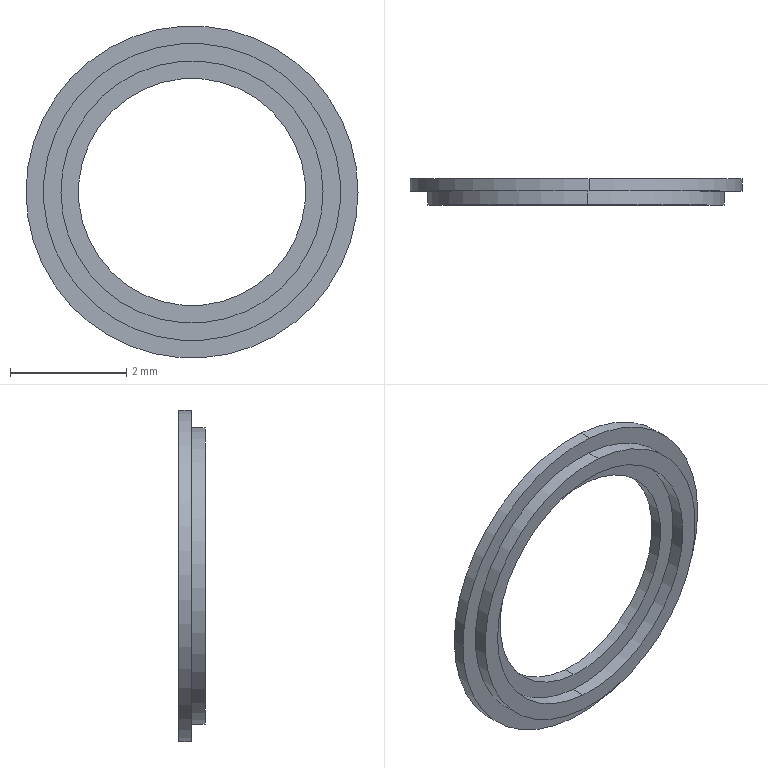Part | STEP file | 2026.6.15-Main Assembly图.sldasm-Part-192 | 1 solid | 12 faces | box 5.7 x 0.45 x 5.7 mm | volume 3.936 mm3 | cylinder 8 | plane 4 | commonest cylinder face diameters 3.9 x2 4.5 x2 5.1 x2 5.7 x2
STEP:
#1=CARTESIAN_POINT('',(-1557.488,1439.564,3405.544));
#2=VERTEX_POINT('',#1);
#3=CARTESIAN_POINT('',(-1557.088,1439.564,3410.628));
#4=VERTEX_POINT('',#3);
#5=CARTESIAN_POINT('',(-1557.288,1439.564,3408.086));
#6=DIRECTION('',(0.,1.,0.));
#7=DIRECTION('',(-0.0785,0.,-0.9969));
#8=AXIS2_PLACEMENT_3D('',#5,#6,#7);
#9=CIRCLE('',#8,2.55);
#10=EDGE_CURVE('',#2,#4,#9,.T.);
#11=ORIENTED_EDGE('',*,*,#10,.F.);
#12=CARTESIAN_POINT('',(-1557.288,1439.564,3408.086));
#13=DIRECTION('',(0.,1.,0.));
#14=DIRECTION('',(-0.0785,0.,-0.9969));
#15=AXIS2_PLACEMENT_3D('',#12,#13,#14);
#16=CIRCLE('',#15,2.55);
#17=EDGE_CURVE('',#4,#2,#16,.T.);
#18=ORIENTED_EDGE('',*,*,#17,.F.);
#19=EDGE_LOOP('',(#11,#18));
#20=FACE_OUTER_BOUND('',#19,.T.);
#21=CARTESIAN_POINT('',(-1557.465,1439.564,3405.843));
#22=VERTEX_POINT('',#21);
#23=CARTESIAN_POINT('',(-1557.112,1439.564,3410.329));
#24=VERTEX_POINT('',#23);
#25=CARTESIAN_POINT('',(-1557.288,1439.564,3408.086));
#26=DIRECTION('',(0.,1.,0.));
#27=DIRECTION('',(-0.0785,0.,-0.9969));
#28=AXIS2_PLACEMENT_3D('',#25,#26,#27);
#29=CIRCLE('',#28,2.25);
#30=EDGE_CURVE('',#22,#24,#29,.T.);
#31=ORIENTED_EDGE('',*,*,#30,.T.);
#32=CARTESIAN_POINT('',(-1557.288,1439.564,3408.086));
#33=DIRECTION('',(0.,1.,0.));
#34=DIRECTION('',(-0.0785,0.,-0.9969));
#35=AXIS2_PLACEMENT_3D('',#32,#33,#34);
#36=CIRCLE('',#35,2.25);
#37=EDGE_CURVE('',#24,#22,#36,.T.);
#38=ORIENTED_EDGE('',*,*,#37,.T.);
#39=EDGE_LOOP('',(#31,#38));
#40=FACE_BOUND('',#39,.T.);
#41=CARTESIAN_POINT('',(-1557.288,1439.564,3410.636));
#42=DIRECTION('',(0.,1.,0.));
#43=DIRECTION('',(1.,0.,0.));
#44=AXIS2_PLACEMENT_3D('',#41,#42,#43);
#45=PLANE('',#44);
#46=ADVANCED_FACE('',(#20,#40),#45,.F.);
#47=CARTESIAN_POINT('',(-1557.112,1439.804,3410.329));
#48=VERTEX_POINT('',#47);
#49=CARTESIAN_POINT('',(-1557.112,1459.814,3410.329));
#50=DIRECTION('',(0.,1.,0.));
#51=VECTOR('',#50,1000.);
#52=LINE('',#49,#51);
#53=EDGE_CURVE('',#24,#48,#52,.T.);
#54=ORIENTED_EDGE('',*,*,#53,.F.);
#55=ORIENTED_EDGE('',*,*,#30,.F.);
#56=CARTESIAN_POINT('',(-1557.465,1439.804,3405.843));
#57=VERTEX_POINT('',#56);
#58=CARTESIAN_POINT('',(-1557.465,1459.814,3405.843));
#59=DIRECTION('',(0.,1.,0.));
#60=VECTOR('',#59,1000.);
#61=LINE('',#58,#60);
#62=EDGE_CURVE('',#22,#57,#61,.T.);
#63=ORIENTED_EDGE('',*,*,#62,.T.);
#64=CARTESIAN_POINT('',(-1557.288,1439.804,3408.086));
#65=DIRECTION('',(0.,1.,0.));
#66=DIRECTION('',(-0.0785,0.,-0.9969));
#67=AXIS2_PLACEMENT_3D('',#64,#65,#66);
#68=CIRCLE('',#67,2.25);
#69=EDGE_CURVE('',#57,#48,#68,.T.);
#70=ORIENTED_EDGE('',*,*,#69,.T.);
#71=EDGE_LOOP('',(#54,#55,#63,#70));
#72=FACE_OUTER_BOUND('',#71,.T.);
#73=CARTESIAN_POINT('',(-1557.288,1459.814,3408.086));
#74=DIRECTION('',(0.,1.,0.));
#75=DIRECTION('',(0.0785,0.,0.9969));
#76=AXIS2_PLACEMENT_3D('',#73,#74,#75);
#77=CYLINDRICAL_SURFACE('',#76,2.25);
#78=ADVANCED_FACE('',(#72),#77,.F.);
#79=CARTESIAN_POINT('',(-1557.088,1439.804,3410.628));
#80=VERTEX_POINT('',#79);
#81=CARTESIAN_POINT('',(-1557.088,1459.814,3410.628));
#82=DIRECTION('',(0.,1.,0.));
#83=VECTOR('',#82,1000.);
#84=LINE('',#81,#83);
#85=EDGE_CURVE('',#4,#80,#84,.T.);
#86=ORIENTED_EDGE('',*,*,#85,.F.);
#87=ORIENTED_EDGE('',*,*,#17,.T.);
#88=CARTESIAN_POINT('',(-1557.488,1439.804,3405.544));
#89=VERTEX_POINT('',#88);
#90=CARTESIAN_POINT('',(-1557.488,1459.814,3405.544));
#91=DIRECTION('',(0.,1.,0.));
#92=VECTOR('',#91,1000.);
#93=LINE('',#90,#92);
#94=EDGE_CURVE('',#2,#89,#93,.T.);
#95=ORIENTED_EDGE('',*,*,#94,.T.);
#96=CARTESIAN_POINT('',(-1557.288,1439.804,3408.086));
#97=DIRECTION('',(0.,-1.,0.));
#98=DIRECTION('',(-0.0785,0.,-0.9969));
#99=AXIS2_PLACEMENT_3D('',#96,#97,#98);
#100=CIRCLE('',#99,2.55);
#101=EDGE_CURVE('',#89,#80,#100,.T.);
#102=ORIENTED_EDGE('',*,*,#101,.T.);
#103=EDGE_LOOP('',(#86,#87,#95,#102));
#104=FACE_OUTER_BOUND('',#103,.T.);
#105=CARTESIAN_POINT('',(-1557.288,1459.814,3408.086));
#106=DIRECTION('',(0.,1.,0.));
#107=DIRECTION('',(0.0785,0.,0.9969));
#108=AXIS2_PLACEMENT_3D('',#105,#106,#107);
#109=CYLINDRICAL_SURFACE('',#108,2.55);
#110=ADVANCED_FACE('',(#104),#109,.T.);
#111=ORIENTED_EDGE('',*,*,#69,.F.);
#112=CARTESIAN_POINT('',(-1557.288,1439.804,3408.086));
#113=DIRECTION('',(0.,1.,0.));
#114=DIRECTION('',(-0.0785,0.,-0.9969));
#115=AXIS2_PLACEMENT_3D('',#112,#113,#114);
#116=CIRCLE('',#115,2.25);
#117=EDGE_CURVE('',#48,#57,#116,.T.);
#118=ORIENTED_EDGE('',*,*,#117,.F.);
#119=EDGE_LOOP('',(#111,#118));
#120=FACE_OUTER_BOUND('',#119,.T.);
#121=CARTESIAN_POINT('',(-1557.441,1439.804,3406.142));
#122=VERTEX_POINT('',#121);
#123=CARTESIAN_POINT('',(-1557.135,1439.804,3410.03));
#124=VERTEX_POINT('',#123);
#125=CARTESIAN_POINT('',(-1557.288,1439.804,3408.086));
#126=DIRECTION('',(0.,1.,0.));
#127=DIRECTION('',(-0.0785,0.,-0.9969));
#128=AXIS2_PLACEMENT_3D('',#125,#126,#127);
#129=CIRCLE('',#128,1.95);
#130=EDGE_CURVE('',#122,#124,#129,.T.);
#131=ORIENTED_EDGE('',*,*,#130,.T.);
#132=CARTESIAN_POINT('',(-1557.288,1439.804,3408.086));
#133=DIRECTION('',(0.,1.,0.));
#134=DIRECTION('',(-0.0785,0.,-0.9969));
#135=AXIS2_PLACEMENT_3D('',#132,#133,#134);
#136=CIRCLE('',#135,1.95);
#137=EDGE_CURVE('',#124,#122,#136,.T.);
#138=ORIENTED_EDGE('',*,*,#137,.T.);
#139=EDGE_LOOP('',(#131,#138));
#140=FACE_BOUND('',#139,.T.);
#141=CARTESIAN_POINT('',(-1557.288,1439.804,3410.336));
#142=DIRECTION('',(0.,1.,0.));
#143=DIRECTION('',(1.,0.,0.));
#144=AXIS2_PLACEMENT_3D('',#141,#142,#143);
#145=PLANE('',#144);
#146=ADVANCED_FACE('',(#120,#140),#145,.F.);
#147=CARTESIAN_POINT('',(-1557.512,1439.804,3405.245));
#148=VERTEX_POINT('',#147);
#149=CARTESIAN_POINT('',(-1557.065,1439.804,3410.928));
#150=VERTEX_POINT('',#149);
#151=CARTESIAN_POINT('',(-1557.288,1439.804,3408.086));
#152=DIRECTION('',(0.,1.,0.));
#153=DIRECTION('',(-0.0785,0.,-0.9969));
#154=AXIS2_PLACEMENT_3D('',#151,#152,#153);
#155=CIRCLE('',#154,2.85);
#156=EDGE_CURVE('',#148,#150,#155,.T.);
#157=ORIENTED_EDGE('',*,*,#156,.F.);
#158=CARTESIAN_POINT('',(-1557.288,1439.804,3408.086));
#159=DIRECTION('',(0.,1.,0.));
#160=DIRECTION('',(-0.0785,0.,-0.9969));
#161=AXIS2_PLACEMENT_3D('',#158,#159,#160);
#162=CIRCLE('',#161,2.85);
#163=EDGE_CURVE('',#150,#148,#162,.T.);
#164=ORIENTED_EDGE('',*,*,#163,.F.);
#165=EDGE_LOOP('',(#157,#164));
#166=FACE_OUTER_BOUND('',#165,.T.);
#167=ORIENTED_EDGE('',*,*,#101,.F.);
#168=CARTESIAN_POINT('',(-1557.288,1439.804,3408.086));
#169=DIRECTION('',(0.,-1.,0.));
#170=DIRECTION('',(-0.0785,0.,-0.9969));
#171=AXIS2_PLACEMENT_3D('',#168,#169,#170);
#172=CIRCLE('',#171,2.55);
#173=EDGE_CURVE('',#80,#89,#172,.T.);
#174=ORIENTED_EDGE('',*,*,#173,.F.);
#175=EDGE_LOOP('',(#167,#174));
#176=FACE_BOUND('',#175,.T.);
#177=CARTESIAN_POINT('',(-1557.288,1439.804,3410.936));
#178=DIRECTION('',(0.,1.,0.));
#179=DIRECTION('',(1.,0.,0.));
#180=AXIS2_PLACEMENT_3D('',#177,#178,#179);
#181=PLANE('',#180);
#182=ADVANCED_FACE('',(#166,#176),#181,.F.);
#183=CARTESIAN_POINT('',(-1557.135,1440.014,3410.03));
#184=VERTEX_POINT('',#183);
#185=CARTESIAN_POINT('',(-1557.135,1459.814,3410.03));
#186=DIRECTION('',(0.,1.,0.));
#187=VECTOR('',#186,1000.);
#188=LINE('',#185,#187);
#189=EDGE_CURVE('',#124,#184,#188,.T.);
#190=ORIENTED_EDGE('',*,*,#189,.F.);
#191=ORIENTED_EDGE('',*,*,#130,.F.);
#192=CARTESIAN_POINT('',(-1557.441,1440.014,3406.142));
#193=VERTEX_POINT('',#192);
#194=CARTESIAN_POINT('',(-1557.441,1459.814,3406.142));
#195=DIRECTION('',(0.,1.,0.));
#196=VECTOR('',#195,1000.);
#197=LINE('',#194,#196);
#198=EDGE_CURVE('',#122,#193,#197,.T.);
#199=ORIENTED_EDGE('',*,*,#198,.T.);
#200=CARTESIAN_POINT('',(-1557.288,1440.014,3408.086));
#201=DIRECTION('',(0.,1.,0.));
#202=DIRECTION('',(-0.0785,0.,-0.9969));
#203=AXIS2_PLACEMENT_3D('',#200,#201,#202);
#204=CIRCLE('',#203,1.95);
#205=EDGE_CURVE('',#193,#184,#204,.T.);
#206=ORIENTED_EDGE('',*,*,#205,.T.);
#207=EDGE_LOOP('',(#190,#191,#199,#206));
#208=FACE_OUTER_BOUND('',#207,.T.);
#209=CARTESIAN_POINT('',(-1557.288,1459.814,3408.086));
#210=DIRECTION('',(0.,1.,0.));
#211=DIRECTION('',(0.0785,0.,0.9969));
#212=AXIS2_PLACEMENT_3D('',#209,#210,#211);
#213=CYLINDRICAL_SURFACE('',#212,1.95);
#214=ADVANCED_FACE('',(#208),#213,.F.);
#215=CARTESIAN_POINT('',(-1557.065,1440.014,3410.928));
#216=VERTEX_POINT('',#215);
#217=CARTESIAN_POINT('',(-1557.065,1459.814,3410.928));
#218=DIRECTION('',(0.,1.,0.));
#219=VECTOR('',#218,1000.);
#220=LINE('',#217,#219);
#221=EDGE_CURVE('',#150,#216,#220,.T.);
#222=ORIENTED_EDGE('',*,*,#221,.F.);
#223=ORIENTED_EDGE('',*,*,#163,.T.);
#224=CARTESIAN_POINT('',(-1557.512,1440.014,3405.245));
#225=VERTEX_POINT('',#224);
#226=CARTESIAN_POINT('',(-1557.512,1459.814,3405.245));
#227=DIRECTION('',(0.,1.,0.));
#228=VECTOR('',#227,1000.);
#229=LINE('',#226,#228);
#230=EDGE_CURVE('',#148,#225,#229,.T.);
#231=ORIENTED_EDGE('',*,*,#230,.T.);
#232=CARTESIAN_POINT('',(-1557.288,1440.014,3408.086));
#233=DIRECTION('',(0.,-1.,0.));
#234=DIRECTION('',(-0.0785,0.,-0.9969));
#235=AXIS2_PLACEMENT_3D('',#232,#233,#234);
#236=CIRCLE('',#235,2.85);
#237=EDGE_CURVE('',#225,#216,#236,.T.);
#238=ORIENTED_EDGE('',*,*,#237,.T.);
#239=EDGE_LOOP('',(#222,#223,#231,#238));
#240=FACE_OUTER_BOUND('',#239,.T.);
#241=CARTESIAN_POINT('',(-1557.288,1459.814,3408.086));
#242=DIRECTION('',(0.,1.,0.));
#243=DIRECTION('',(0.0785,0.,0.9969));
#244=AXIS2_PLACEMENT_3D('',#241,#242,#243);
#245=CYLINDRICAL_SURFACE('',#244,2.85);
#246=ADVANCED_FACE('',(#240),#245,.T.);
#247=ORIENTED_EDGE('',*,*,#237,.F.);
#248=CARTESIAN_POINT('',(-1557.288,1440.014,3408.086));
#249=DIRECTION('',(0.,-1.,0.));
#250=DIRECTION('',(-0.0785,0.,-0.9969));
#251=AXIS2_PLACEMENT_3D('',#248,#249,#250);
#252=CIRCLE('',#251,2.85);
#253=EDGE_CURVE('',#216,#225,#252,.T.);
#254=ORIENTED_EDGE('',*,*,#253,.F.);
#255=EDGE_LOOP('',(#247,#254));
#256=FACE_OUTER_BOUND('',#255,.T.);
#257=ORIENTED_EDGE('',*,*,#205,.F.);
#258=CARTESIAN_POINT('',(-1557.288,1440.014,3408.086));
#259=DIRECTION('',(0.,1.,0.));
#260=DIRECTION('',(-0.0785,0.,-0.9969));
#261=AXIS2_PLACEMENT_3D('',#258,#259,#260);
#262=CIRCLE('',#261,1.95);
#263=EDGE_CURVE('',#184,#193,#262,.T.);
#264=ORIENTED_EDGE('',*,*,#263,.F.);
#265=EDGE_LOOP('',(#257,#264));
#266=FACE_BOUND('',#265,.T.);
#267=CARTESIAN_POINT('',(-1557.288,1440.014,3410.036));
#268=DIRECTION('',(0.,-1.,0.));
#269=DIRECTION('',(0.,0.,-1.));
#270=AXIS2_PLACEMENT_3D('',#267,#268,#269);
#271=PLANE('',#270);
#272=ADVANCED_FACE('',(#256,#266),#271,.F.);
#273=ORIENTED_EDGE('',*,*,#37,.F.);
#274=ORIENTED_EDGE('',*,*,#53,.T.);
#275=ORIENTED_EDGE('',*,*,#117,.T.);
#276=ORIENTED_EDGE('',*,*,#62,.F.);
#277=EDGE_LOOP('',(#273,#274,#275,#276));
#278=FACE_OUTER_BOUND('',#277,.T.);
#279=CARTESIAN_POINT('',(-1557.288,1459.814,3408.086));
#280=DIRECTION('',(0.,1.,0.));
#281=DIRECTION('',(0.0785,0.,0.9969));
#282=AXIS2_PLACEMENT_3D('',#279,#280,#281);
#283=CYLINDRICAL_SURFACE('',#282,2.25);
#284=ADVANCED_FACE('',(#278),#283,.F.);
#285=ORIENTED_EDGE('',*,*,#10,.T.);
#286=ORIENTED_EDGE('',*,*,#85,.T.);
#287=ORIENTED_EDGE('',*,*,#173,.T.);
#288=ORIENTED_EDGE('',*,*,#94,.F.);
#289=EDGE_LOOP('',(#285,#286,#287,#288));
#290=FACE_OUTER_BOUND('',#289,.T.);
#291=CARTESIAN_POINT('',(-1557.288,1459.814,3408.086));
#292=DIRECTION('',(0.,1.,0.));
#293=DIRECTION('',(0.0785,0.,0.9969));
#294=AXIS2_PLACEMENT_3D('',#291,#292,#293);
#295=CYLINDRICAL_SURFACE('',#294,2.55);
#296=ADVANCED_FACE('',(#290),#295,.T.);
#297=ORIENTED_EDGE('',*,*,#137,.F.);
#298=ORIENTED_EDGE('',*,*,#189,.T.);
#299=ORIENTED_EDGE('',*,*,#263,.T.);
#300=ORIENTED_EDGE('',*,*,#198,.F.);
#301=EDGE_LOOP('',(#297,#298,#299,#300));
#302=FACE_OUTER_BOUND('',#301,.T.);
#303=CARTESIAN_POINT('',(-1557.288,1459.814,3408.086));
#304=DIRECTION('',(0.,1.,0.));
#305=DIRECTION('',(0.0785,0.,0.9969));
#306=AXIS2_PLACEMENT_3D('',#303,#304,#305);
#307=CYLINDRICAL_SURFACE('',#306,1.95);
#308=ADVANCED_FACE('',(#302),#307,.F.);
#309=ORIENTED_EDGE('',*,*,#156,.T.);
#310=ORIENTED_EDGE('',*,*,#221,.T.);
#311=ORIENTED_EDGE('',*,*,#253,.T.);
#312=ORIENTED_EDGE('',*,*,#230,.F.);
#313=EDGE_LOOP('',(#309,#310,#311,#312));
#314=FACE_OUTER_BOUND('',#313,.T.);
#315=CARTESIAN_POINT('',(-1557.288,1459.814,3408.086));
#316=DIRECTION('',(0.,1.,0.));
#317=DIRECTION('',(0.0785,0.,0.9969));
#318=AXIS2_PLACEMENT_3D('',#315,#316,#317);
#319=CYLINDRICAL_SURFACE('',#318,2.85);
#320=ADVANCED_FACE('',(#314),#319,.T.);
#321=CLOSED_SHELL('',(#46,#78,#110,#146,#182,#214,#246,#272,#284,#296,#308,#320));
#322=MANIFOLD_SOLID_BREP('',#321);
#323=CARTESIAN_POINT('',(0.,0.,0.));
#324=DIRECTION('',(0.,0.,1.));
#325=DIRECTION('',(1.,0.,0.));
#326=AXIS2_PLACEMENT_3D('',#323,#324,#325);
#327=(LENGTH_UNIT()NAMED_UNIT(*)SI_UNIT(.MILLI.,.METRE.));
#328=UNCERTAINTY_MEASURE_WITH_UNIT(LENGTH_MEASURE(0.00001),#327,'','');
#329=(NAMED_UNIT(*)PLANE_ANGLE_UNIT()SI_UNIT($,.RADIAN.));
#330=(NAMED_UNIT(*)SI_UNIT($,.STERADIAN.)SOLID_ANGLE_UNIT());
#331=(GEOMETRIC_REPRESENTATION_CONTEXT(3)GLOBAL_UNCERTAINTY_ASSIGNED_CONTEXT((#328))GLOBAL_UNIT_ASSIGNED_CONTEXT((#327,#329,#330))REPRESENTATION_CONTEXT('',''));
#332=ADVANCED_BREP_SHAPE_REPRESENTATION('',(#322,#326),#331);